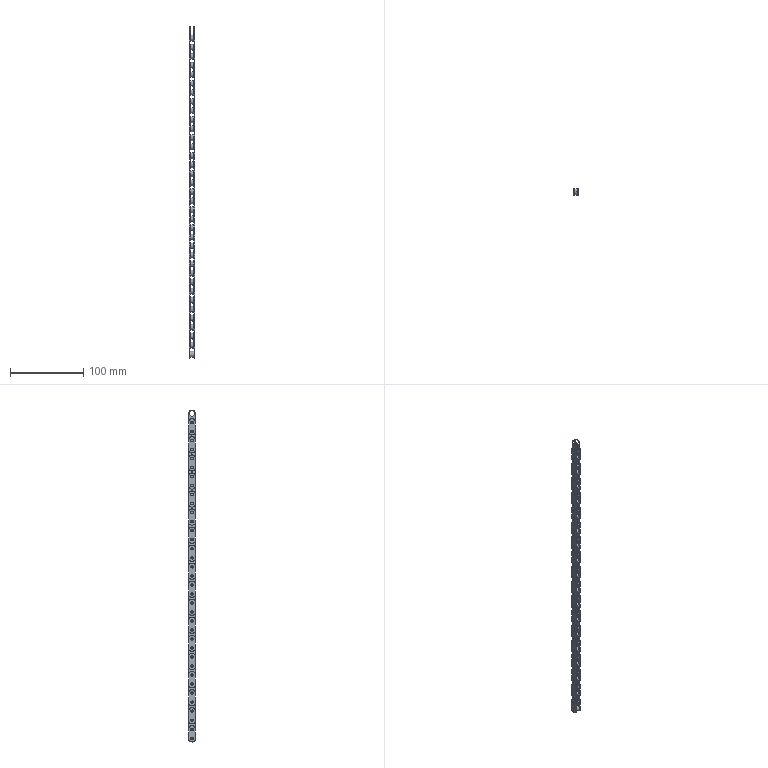Part | STEP file | 17 Chain Links v2 | 18 solids | 1188 faces | box 8 x 10 x 452.3 mm | volume 19900 mm3 | cylinder 576 | plane 360 | torus 252 | commonest cylinder face diameters 3 x144 8 x144 9 x108 10 x108 0.4 x72